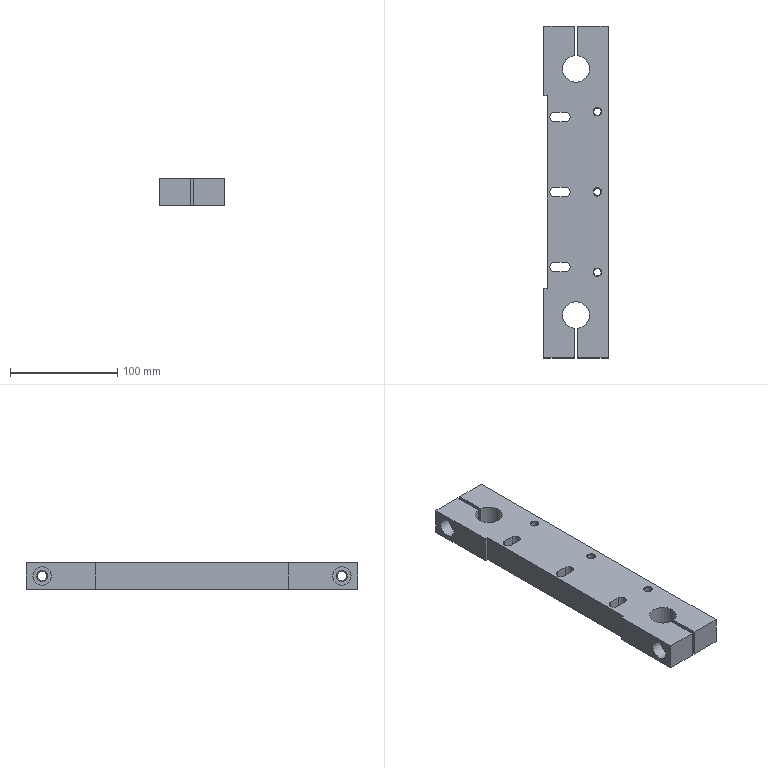Part | STEP file | YBQDJ-QD-3 | 1 solid | 51 faces | box 60 x 310 x 25 mm | volume 397510 mm3 | plane 24 | cylinder 17 | cone 10 | commonest cylinder face diameters 9 x6 6.8 x3 8.5 x2 10.5 x2 17 x2 25.02 x2